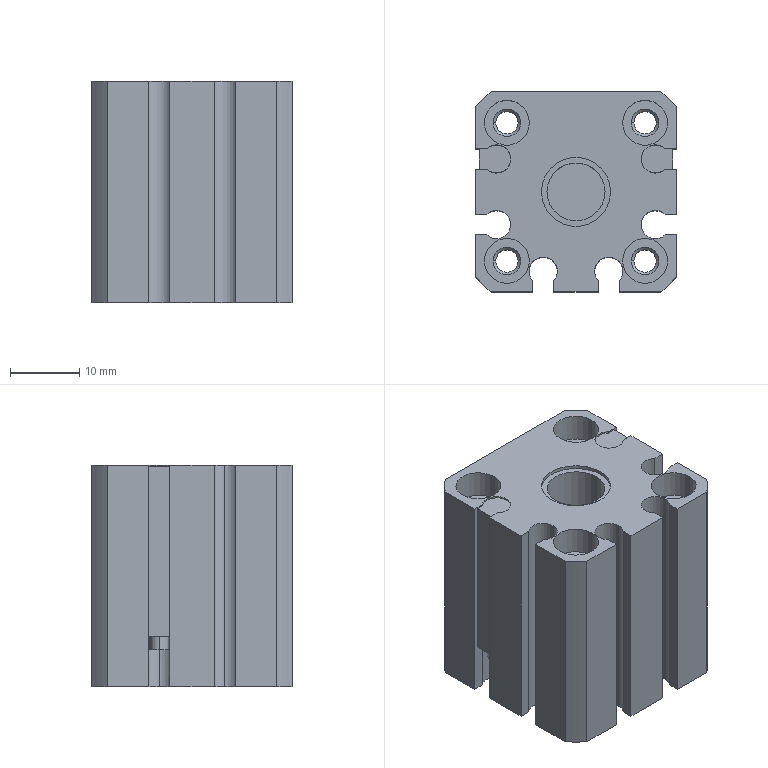Part | STEP file | 11-Body_A_CDQSB16_10D_A93_0_11 | 1 solid | 152 faces | box 29 x 29 x 32 mm | volume 21093 mm3 | cylinder 72 | plane 60 | cone 20 | commonest cylinder face diameters 3.24 x16 6.5 x16 4.1 x12 3.5 x8 2.7 x4 4 x4